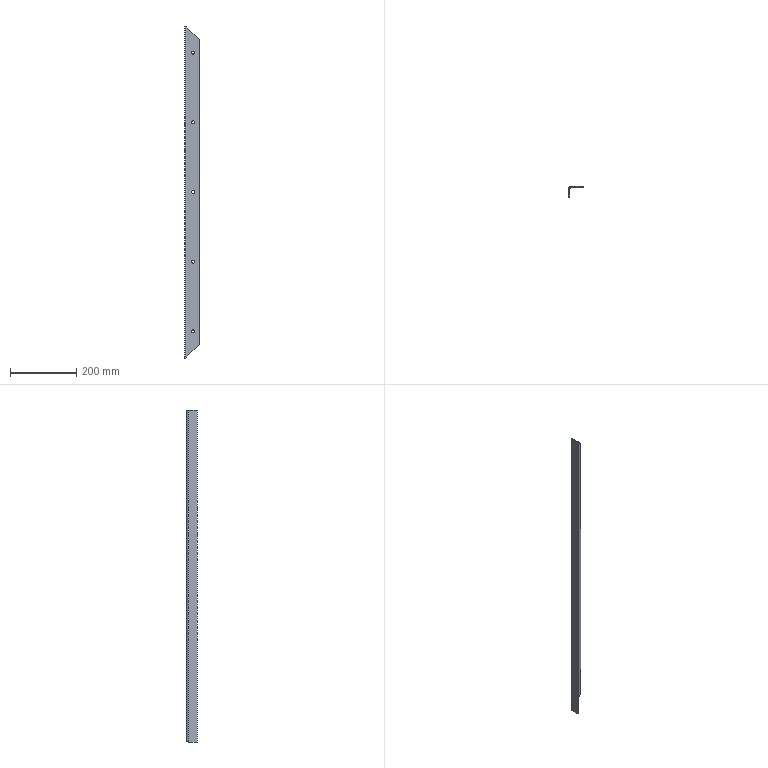Part | STEP file | 750038391 | 1 solid | 24 faces | box 43 x 33 x 1000 mm | volume 207432 mm3 | cylinder 12 | plane 10 | spline 2 | commonest cylinder face diameters 9 x10 6 x1 12 x1
STEP:
#1=CARTESIAN_POINT('',(22.,0.,415.5));
#2=VERTEX_POINT('',#1);
#3=CARTESIAN_POINT('',(22.,0.,424.5));
#4=VERTEX_POINT('',#3);
#5=CARTESIAN_POINT('',(22.,0.,420.));
#6=DIRECTION('',(0.,1.,0.));
#7=DIRECTION('',(0.,0.,1.));
#8=AXIS2_PLACEMENT_3D('',#5,#6,#7);
#9=CIRCLE('',#8,4.5);
#10=EDGE_CURVE('',#2,#4,#9,.T.);
#11=ORIENTED_EDGE('',*,*,#10,.F.);
#12=CARTESIAN_POINT('',(22.,3.,415.5));
#13=VERTEX_POINT('',#12);
#14=CARTESIAN_POINT('',(22.,-998.468,415.5));
#15=DIRECTION('',(0.,1.,0.));
#16=VECTOR('',#15,1000.);
#17=LINE('',#14,#16);
#18=EDGE_CURVE('',#2,#13,#17,.T.);
#19=ORIENTED_EDGE('',*,*,#18,.T.);
#20=CARTESIAN_POINT('',(22.,3.,424.5));
#21=VERTEX_POINT('',#20);
#22=CARTESIAN_POINT('',(22.,3.,420.));
#23=DIRECTION('',(0.,1.,0.));
#24=DIRECTION('',(0.,0.,1.));
#25=AXIS2_PLACEMENT_3D('',#22,#23,#24);
#26=CIRCLE('',#25,4.5);
#27=EDGE_CURVE('',#13,#21,#26,.T.);
#28=ORIENTED_EDGE('',*,*,#27,.T.);
#29=CARTESIAN_POINT('',(22.,-998.468,424.5));
#30=DIRECTION('',(0.,1.,0.));
#31=VECTOR('',#30,1000.);
#32=LINE('',#29,#31);
#33=EDGE_CURVE('',#4,#21,#32,.T.);
#34=ORIENTED_EDGE('',*,*,#33,.F.);
#35=EDGE_LOOP('',(#11,#19,#28,#34));
#36=FACE_OUTER_BOUND('',#35,.T.);
#37=CARTESIAN_POINT('',(22.,-998.468,420.));
#38=DIRECTION('',(0.,1.,0.));
#39=DIRECTION('',(0.,0.,1.));
#40=AXIS2_PLACEMENT_3D('',#37,#38,#39);
#41=CYLINDRICAL_SURFACE('',#40,4.5);
#42=ADVANCED_FACE('',(#36),#41,.F.);
#43=CARTESIAN_POINT('',(22.,0.,205.5));
#44=VERTEX_POINT('',#43);
#45=CARTESIAN_POINT('',(22.,0.,214.5));
#46=VERTEX_POINT('',#45);
#47=CARTESIAN_POINT('',(22.,0.,210.));
#48=DIRECTION('',(0.,1.,0.));
#49=DIRECTION('',(0.,0.,1.));
#50=AXIS2_PLACEMENT_3D('',#47,#48,#49);
#51=CIRCLE('',#50,4.5);
#52=EDGE_CURVE('',#44,#46,#51,.T.);
#53=ORIENTED_EDGE('',*,*,#52,.F.);
#54=CARTESIAN_POINT('',(22.,3.,205.5));
#55=VERTEX_POINT('',#54);
#56=CARTESIAN_POINT('',(22.,-998.468,205.5));
#57=DIRECTION('',(0.,1.,0.));
#58=VECTOR('',#57,1000.);
#59=LINE('',#56,#58);
#60=EDGE_CURVE('',#44,#55,#59,.T.);
#61=ORIENTED_EDGE('',*,*,#60,.T.);
#62=CARTESIAN_POINT('',(22.,3.,214.5));
#63=VERTEX_POINT('',#62);
#64=CARTESIAN_POINT('',(22.,3.,210.));
#65=DIRECTION('',(0.,1.,0.));
#66=DIRECTION('',(0.,0.,1.));
#67=AXIS2_PLACEMENT_3D('',#64,#65,#66);
#68=CIRCLE('',#67,4.5);
#69=EDGE_CURVE('',#55,#63,#68,.T.);
#70=ORIENTED_EDGE('',*,*,#69,.T.);
#71=CARTESIAN_POINT('',(22.,-998.468,214.5));
#72=DIRECTION('',(0.,1.,0.));
#73=VECTOR('',#72,1000.);
#74=LINE('',#71,#73);
#75=EDGE_CURVE('',#46,#63,#74,.T.);
#76=ORIENTED_EDGE('',*,*,#75,.F.);
#77=EDGE_LOOP('',(#53,#61,#70,#76));
#78=FACE_OUTER_BOUND('',#77,.T.);
#79=CARTESIAN_POINT('',(22.,-998.468,210.));
#80=DIRECTION('',(0.,1.,0.));
#81=DIRECTION('',(0.,0.,1.));
#82=AXIS2_PLACEMENT_3D('',#79,#80,#81);
#83=CYLINDRICAL_SURFACE('',#82,4.5);
#84=ADVANCED_FACE('',(#78),#83,.F.);
#85=CARTESIAN_POINT('',(22.,0.,-4.5));
#86=VERTEX_POINT('',#85);
#87=CARTESIAN_POINT('',(22.,0.,4.5));
#88=VERTEX_POINT('',#87);
#89=CARTESIAN_POINT('',(22.,0.,0.));
#90=DIRECTION('',(0.,1.,0.));
#91=DIRECTION('',(0.,0.,1.));
#92=AXIS2_PLACEMENT_3D('',#89,#90,#91);
#93=CIRCLE('',#92,4.5);
#94=EDGE_CURVE('',#86,#88,#93,.T.);
#95=ORIENTED_EDGE('',*,*,#94,.F.);
#96=CARTESIAN_POINT('',(22.,3.,-4.5));
#97=VERTEX_POINT('',#96);
#98=CARTESIAN_POINT('',(22.,-998.468,-4.5));
#99=DIRECTION('',(0.,1.,0.));
#100=VECTOR('',#99,1000.);
#101=LINE('',#98,#100);
#102=EDGE_CURVE('',#86,#97,#101,.T.);
#103=ORIENTED_EDGE('',*,*,#102,.T.);
#104=CARTESIAN_POINT('',(22.,3.,4.5));
#105=VERTEX_POINT('',#104);
#106=CARTESIAN_POINT('',(22.,3.,0.));
#107=DIRECTION('',(0.,1.,0.));
#108=DIRECTION('',(0.,0.,1.));
#109=AXIS2_PLACEMENT_3D('',#106,#107,#108);
#110=CIRCLE('',#109,4.5);
#111=EDGE_CURVE('',#97,#105,#110,.T.);
#112=ORIENTED_EDGE('',*,*,#111,.T.);
#113=CARTESIAN_POINT('',(22.,-998.468,4.5));
#114=DIRECTION('',(0.,1.,0.));
#115=VECTOR('',#114,1000.);
#116=LINE('',#113,#115);
#117=EDGE_CURVE('',#88,#105,#116,.T.);
#118=ORIENTED_EDGE('',*,*,#117,.F.);
#119=EDGE_LOOP('',(#95,#103,#112,#118));
#120=FACE_OUTER_BOUND('',#119,.T.);
#121=CARTESIAN_POINT('',(22.,-998.468,0.));
#122=DIRECTION('',(0.,1.,0.));
#123=DIRECTION('',(0.,0.,1.));
#124=AXIS2_PLACEMENT_3D('',#121,#122,#123);
#125=CYLINDRICAL_SURFACE('',#124,4.5);
#126=ADVANCED_FACE('',(#120),#125,.F.);
#127=CARTESIAN_POINT('',(22.,0.,-214.5));
#128=VERTEX_POINT('',#127);
#129=CARTESIAN_POINT('',(22.,0.,-205.5));
#130=VERTEX_POINT('',#129);
#131=CARTESIAN_POINT('',(22.,0.,-210.));
#132=DIRECTION('',(0.,1.,0.));
#133=DIRECTION('',(0.,0.,1.));
#134=AXIS2_PLACEMENT_3D('',#131,#132,#133);
#135=CIRCLE('',#134,4.5);
#136=EDGE_CURVE('',#128,#130,#135,.T.);
#137=ORIENTED_EDGE('',*,*,#136,.F.);
#138=CARTESIAN_POINT('',(22.,3.,-214.5));
#139=VERTEX_POINT('',#138);
#140=CARTESIAN_POINT('',(22.,-998.468,-214.5));
#141=DIRECTION('',(0.,1.,0.));
#142=VECTOR('',#141,1000.);
#143=LINE('',#140,#142);
#144=EDGE_CURVE('',#128,#139,#143,.T.);
#145=ORIENTED_EDGE('',*,*,#144,.T.);
#146=CARTESIAN_POINT('',(22.,3.,-205.5));
#147=VERTEX_POINT('',#146);
#148=CARTESIAN_POINT('',(22.,3.,-210.));
#149=DIRECTION('',(0.,1.,0.));
#150=DIRECTION('',(0.,0.,1.));
#151=AXIS2_PLACEMENT_3D('',#148,#149,#150);
#152=CIRCLE('',#151,4.5);
#153=EDGE_CURVE('',#139,#147,#152,.T.);
#154=ORIENTED_EDGE('',*,*,#153,.T.);
#155=CARTESIAN_POINT('',(22.,-998.468,-205.5));
#156=DIRECTION('',(0.,1.,0.));
#157=VECTOR('',#156,1000.);
#158=LINE('',#155,#157);
#159=EDGE_CURVE('',#130,#147,#158,.T.);
#160=ORIENTED_EDGE('',*,*,#159,.F.);
#161=EDGE_LOOP('',(#137,#145,#154,#160));
#162=FACE_OUTER_BOUND('',#161,.T.);
#163=CARTESIAN_POINT('',(22.,-998.468,-210.));
#164=DIRECTION('',(0.,1.,0.));
#165=DIRECTION('',(0.,0.,1.));
#166=AXIS2_PLACEMENT_3D('',#163,#164,#165);
#167=CYLINDRICAL_SURFACE('',#166,4.5);
#168=ADVANCED_FACE('',(#162),#167,.F.);
#169=CARTESIAN_POINT('',(22.,0.,-424.5));
#170=VERTEX_POINT('',#169);
#171=CARTESIAN_POINT('',(22.,0.,-415.5));
#172=VERTEX_POINT('',#171);
#173=CARTESIAN_POINT('',(22.,0.,-420.));
#174=DIRECTION('',(0.,1.,0.));
#175=DIRECTION('',(0.,0.,1.));
#176=AXIS2_PLACEMENT_3D('',#173,#174,#175);
#177=CIRCLE('',#176,4.5);
#178=EDGE_CURVE('',#170,#172,#177,.T.);
#179=ORIENTED_EDGE('',*,*,#178,.F.);
#180=CARTESIAN_POINT('',(22.,3.,-424.5));
#181=VERTEX_POINT('',#180);
#182=CARTESIAN_POINT('',(22.,-998.468,-424.5));
#183=DIRECTION('',(0.,1.,0.));
#184=VECTOR('',#183,1000.);
#185=LINE('',#182,#184);
#186=EDGE_CURVE('',#170,#181,#185,.T.);
#187=ORIENTED_EDGE('',*,*,#186,.T.);
#188=CARTESIAN_POINT('',(22.,3.,-415.5));
#189=VERTEX_POINT('',#188);
#190=CARTESIAN_POINT('',(22.,3.,-420.));
#191=DIRECTION('',(0.,1.,0.));
#192=DIRECTION('',(0.,0.,1.));
#193=AXIS2_PLACEMENT_3D('',#190,#191,#192);
#194=CIRCLE('',#193,4.5);
#195=EDGE_CURVE('',#181,#189,#194,.T.);
#196=ORIENTED_EDGE('',*,*,#195,.T.);
#197=CARTESIAN_POINT('',(22.,-998.468,-415.5));
#198=DIRECTION('',(0.,1.,0.));
#199=VECTOR('',#198,1000.);
#200=LINE('',#197,#199);
#201=EDGE_CURVE('',#172,#189,#200,.T.);
#202=ORIENTED_EDGE('',*,*,#201,.F.);
#203=EDGE_LOOP('',(#179,#187,#196,#202));
#204=FACE_OUTER_BOUND('',#203,.T.);
#205=CARTESIAN_POINT('',(22.,-998.468,-420.));
#206=DIRECTION('',(0.,1.,0.));
#207=DIRECTION('',(0.,0.,1.));
#208=AXIS2_PLACEMENT_3D('',#205,#206,#207);
#209=CYLINDRICAL_SURFACE('',#208,4.5);
#210=ADVANCED_FACE('',(#204),#209,.F.);
#211=CARTESIAN_POINT('',(40.,3.,-460.));
#212=VERTEX_POINT('',#211);
#213=CARTESIAN_POINT('',(40.,3.,460.));
#214=VERTEX_POINT('',#213);
#215=CARTESIAN_POINT('',(40.,3.,500.));
#216=DIRECTION('',(0.,0.,1.));
#217=VECTOR('',#216,1000.);
#218=LINE('',#215,#217);
#219=EDGE_CURVE('',#212,#214,#218,.T.);
#220=ORIENTED_EDGE('',*,*,#219,.F.);
#221=CARTESIAN_POINT('',(3.,3.,-497.));
#222=VERTEX_POINT('',#221);
#223=CARTESIAN_POINT('',(3.,3.,-497.));
#224=DIRECTION('',(0.7071,0.,0.7071));
#225=VECTOR('',#224,1000.);
#226=LINE('',#223,#225);
#227=EDGE_CURVE('',#222,#212,#226,.T.);
#228=ORIENTED_EDGE('',*,*,#227,.F.);
#229=CARTESIAN_POINT('',(3.,3.,497.));
#230=VERTEX_POINT('',#229);
#231=CARTESIAN_POINT('',(3.,3.,500.));
#232=DIRECTION('',(0.,0.,-1.));
#233=VECTOR('',#232,1000.);
#234=LINE('',#231,#233);
#235=EDGE_CURVE('',#230,#222,#234,.T.);
#236=ORIENTED_EDGE('',*,*,#235,.F.);
#237=CARTESIAN_POINT('',(40.,3.,460.));
#238=DIRECTION('',(-0.7071,0.,0.7071));
#239=VECTOR('',#238,1000.);
#240=LINE('',#237,#239);
#241=EDGE_CURVE('',#214,#230,#240,.T.);
#242=ORIENTED_EDGE('',*,*,#241,.F.);
#243=EDGE_LOOP('',(#220,#228,#236,#242));
#244=FACE_OUTER_BOUND('',#243,.T.);
#245=CARTESIAN_POINT('',(22.,3.,420.));
#246=DIRECTION('',(0.,1.,0.));
#247=DIRECTION('',(0.,0.,1.));
#248=AXIS2_PLACEMENT_3D('',#245,#246,#247);
#249=CIRCLE('',#248,4.5);
#250=EDGE_CURVE('',#21,#13,#249,.T.);
#251=ORIENTED_EDGE('',*,*,#250,.F.);
#252=ORIENTED_EDGE('',*,*,#27,.F.);
#253=EDGE_LOOP('',(#251,#252));
#254=FACE_BOUND('',#253,.T.);
#255=CARTESIAN_POINT('',(22.,3.,210.));
#256=DIRECTION('',(0.,1.,0.));
#257=DIRECTION('',(0.,0.,1.));
#258=AXIS2_PLACEMENT_3D('',#255,#256,#257);
#259=CIRCLE('',#258,4.5);
#260=EDGE_CURVE('',#63,#55,#259,.T.);
#261=ORIENTED_EDGE('',*,*,#260,.F.);
#262=ORIENTED_EDGE('',*,*,#69,.F.);
#263=EDGE_LOOP('',(#261,#262));
#264=FACE_BOUND('',#263,.T.);
#265=CARTESIAN_POINT('',(22.,3.,0.));
#266=DIRECTION('',(0.,1.,0.));
#267=DIRECTION('',(0.,0.,1.));
#268=AXIS2_PLACEMENT_3D('',#265,#266,#267);
#269=CIRCLE('',#268,4.5);
#270=EDGE_CURVE('',#105,#97,#269,.T.);
#271=ORIENTED_EDGE('',*,*,#270,.F.);
#272=ORIENTED_EDGE('',*,*,#111,.F.);
#273=EDGE_LOOP('',(#271,#272));
#274=FACE_BOUND('',#273,.T.);
#275=CARTESIAN_POINT('',(22.,3.,-210.));
#276=DIRECTION('',(0.,1.,0.));
#277=DIRECTION('',(0.,0.,1.));
#278=AXIS2_PLACEMENT_3D('',#275,#276,#277);
#279=CIRCLE('',#278,4.5);
#280=EDGE_CURVE('',#147,#139,#279,.T.);
#281=ORIENTED_EDGE('',*,*,#280,.F.);
#282=ORIENTED_EDGE('',*,*,#153,.F.);
#283=EDGE_LOOP('',(#281,#282));
#284=FACE_BOUND('',#283,.T.);
#285=CARTESIAN_POINT('',(22.,3.,-420.));
#286=DIRECTION('',(0.,1.,0.));
#287=DIRECTION('',(0.,0.,1.));
#288=AXIS2_PLACEMENT_3D('',#285,#286,#287);
#289=CIRCLE('',#288,4.5);
#290=EDGE_CURVE('',#189,#181,#289,.T.);
#291=ORIENTED_EDGE('',*,*,#290,.F.);
#292=ORIENTED_EDGE('',*,*,#195,.F.);
#293=EDGE_LOOP('',(#291,#292));
#294=FACE_BOUND('',#293,.T.);
#295=CARTESIAN_POINT('',(40.,3.,500.));
#296=DIRECTION('',(0.,-1.,0.));
#297=DIRECTION('',(0.,0.,-1.));
#298=AXIS2_PLACEMENT_3D('',#295,#296,#297);
#299=PLANE('',#298);
#300=ADVANCED_FACE('',(#244,#254,#264,#274,#284,#294),#299,.F.);
#301=CARTESIAN_POINT('',(40.,0.,460.));
#302=VERTEX_POINT('',#301);
#303=CARTESIAN_POINT('',(40.,0.,460.));
#304=DIRECTION('',(0.,1.,0.));
#305=VECTOR('',#304,1000.);
#306=LINE('',#303,#305);
#307=EDGE_CURVE('',#302,#214,#306,.T.);
#308=ORIENTED_EDGE('',*,*,#307,.T.);
#309=ORIENTED_EDGE('',*,*,#241,.T.);
#310=CARTESIAN_POINT('',(3.,0.,497.));
#311=VERTEX_POINT('',#310);
#312=CARTESIAN_POINT('',(3.,0.,497.));
#313=DIRECTION('',(0.,-1.,0.));
#314=VECTOR('',#313,1000.);
#315=LINE('',#312,#314);
#316=EDGE_CURVE('',#230,#311,#315,.T.);
#317=ORIENTED_EDGE('',*,*,#316,.T.);
#318=CARTESIAN_POINT('',(20.,0.,480.));
#319=DIRECTION('',(0.7071,0.,-0.7071));
#320=VECTOR('',#319,1000.);
#321=LINE('',#318,#320);
#322=EDGE_CURVE('',#311,#302,#321,.T.);
#323=ORIENTED_EDGE('',*,*,#322,.T.);
#324=EDGE_LOOP('',(#308,#309,#317,#323));
#325=FACE_OUTER_BOUND('',#324,.T.);
#326=CARTESIAN_POINT('',(20.,0.,480.));
#327=DIRECTION('',(0.7071,0.,0.7071));
#328=DIRECTION('',(0.7071,0.,-0.7071));
#329=AXIS2_PLACEMENT_3D('',#326,#327,#328);
#330=PLANE('',#329);
#331=ADVANCED_FACE('',(#325),#330,.T.);
#332=ORIENTED_EDGE('',*,*,#307,.F.);
#333=CARTESIAN_POINT('',(40.,0.,-460.));
#334=VERTEX_POINT('',#333);
#335=CARTESIAN_POINT('',(40.,0.,500.));
#336=DIRECTION('',(0.,0.,1.));
#337=VECTOR('',#336,1000.);
#338=LINE('',#335,#337);
#339=EDGE_CURVE('',#334,#302,#338,.T.);
#340=ORIENTED_EDGE('',*,*,#339,.F.);
#341=CARTESIAN_POINT('',(40.,0.,-460.));
#342=DIRECTION('',(0.,-1.,0.));
#343=VECTOR('',#342,1000.);
#344=LINE('',#341,#343);
#345=EDGE_CURVE('',#212,#334,#344,.T.);
#346=ORIENTED_EDGE('',*,*,#345,.F.);
#347=ORIENTED_EDGE('',*,*,#219,.T.);
#348=EDGE_LOOP('',(#332,#340,#346,#347));
#349=FACE_OUTER_BOUND('',#348,.T.);
#350=CARTESIAN_POINT('',(40.,0.,500.));
#351=DIRECTION('',(-1.,0.,0.));
#352=DIRECTION('',(0.,0.,1.));
#353=AXIS2_PLACEMENT_3D('',#350,#351,#352);
#354=PLANE('',#353);
#355=ADVANCED_FACE('',(#349),#354,.F.);
#356=CARTESIAN_POINT('',(3.,0.,-497.));
#357=VERTEX_POINT('',#356);
#358=CARTESIAN_POINT('',(3.,0.,-497.));
#359=DIRECTION('',(0.,1.,0.));
#360=VECTOR('',#359,1000.);
#361=LINE('',#358,#360);
#362=EDGE_CURVE('',#357,#222,#361,.T.);
#363=ORIENTED_EDGE('',*,*,#362,.T.);
#364=ORIENTED_EDGE('',*,*,#227,.T.);
#365=ORIENTED_EDGE('',*,*,#345,.T.);
#366=CARTESIAN_POINT('',(520.,0.,20.));
#367=DIRECTION('',(-0.7071,0.,-0.7071));
#368=VECTOR('',#367,1000.);
#369=LINE('',#366,#368);
#370=EDGE_CURVE('',#334,#357,#369,.T.);
#371=ORIENTED_EDGE('',*,*,#370,.T.);
#372=EDGE_LOOP('',(#363,#364,#365,#371));
#373=FACE_OUTER_BOUND('',#372,.T.);
#374=CARTESIAN_POINT('',(520.,0.,20.));
#375=DIRECTION('',(0.7071,0.,-0.7071));
#376=DIRECTION('',(-0.7071,0.,-0.7071));
#377=AXIS2_PLACEMENT_3D('',#374,#375,#376);
#378=PLANE('',#377);
#379=ADVANCED_FACE('',(#373),#378,.T.);
#380=CARTESIAN_POINT('',(-3.,-3.,-500.));
#381=VERTEX_POINT('',#380);
#382=CARTESIAN_POINT('',(3.,3.,-497.));
#383=CARTESIAN_POINT('',(-1.,3.,-499.));
#384=CARTESIAN_POINT('',(-3.,0.,-500.));
#385=CARTESIAN_POINT('',(-3.,-3.,-500.));
#386=(BOUNDED_CURVE()B_SPLINE_CURVE(3,(#382,#383,#384,#385),.UNSPECIFIED.,.F.,.T.)B_SPLINE_CURVE_WITH_KNOTS((4,4),(0.,0.009933),.UNSPECIFIED.)CURVE()GEOMETRIC_REPRESENTATION_ITEM()RATIONAL_B_SPLINE_CURVE((0.5,0.5,0.6667,1.))REPRESENTATION_ITEM(''));
#387=EDGE_CURVE('',#222,#381,#386,.T.);
#388=ORIENTED_EDGE('',*,*,#387,.T.);
#389=CARTESIAN_POINT('',(-3.,-3.,500.));
#390=VERTEX_POINT('',#389);
#391=CARTESIAN_POINT('',(-3.,-3.,500.));
#392=DIRECTION('',(0.,0.,1.));
#393=VECTOR('',#392,1000.);
#394=LINE('',#391,#393);
#395=EDGE_CURVE('',#381,#390,#394,.T.);
#396=ORIENTED_EDGE('',*,*,#395,.T.);
#397=CARTESIAN_POINT('',(-3.,-3.,500.));
#398=CARTESIAN_POINT('',(-3.,0.,500.));
#399=CARTESIAN_POINT('',(-1.,3.,499.));
#400=CARTESIAN_POINT('',(3.,3.,497.));
#401=(BOUNDED_CURVE()B_SPLINE_CURVE(3,(#397,#398,#399,#400),.UNSPECIFIED.,.F.,.T.)B_SPLINE_CURVE_WITH_KNOTS((4,4),(0.,0.009979),.UNSPECIFIED.)CURVE()GEOMETRIC_REPRESENTATION_ITEM()RATIONAL_B_SPLINE_CURVE((1.,0.6667,0.5,0.5))REPRESENTATION_ITEM(''));
#402=EDGE_CURVE('',#390,#230,#401,.T.);
#403=ORIENTED_EDGE('',*,*,#402,.T.);
#404=ORIENTED_EDGE('',*,*,#235,.T.);
#405=EDGE_LOOP('',(#388,#396,#403,#404));
#406=FACE_OUTER_BOUND('',#405,.T.);
#407=CARTESIAN_POINT('',(3.,-3.,500.));
#408=DIRECTION('',(0.,0.,-1.));
#409=DIRECTION('',(-1.,0.,0.));
#410=AXIS2_PLACEMENT_3D('',#407,#408,#409);
#411=CYLINDRICAL_SURFACE('',#410,6.);
#412=ADVANCED_FACE('',(#406),#411,.T.);
#413=ORIENTED_EDGE('',*,*,#18,.F.);
#414=CARTESIAN_POINT('',(22.,0.,420.));
#415=DIRECTION('',(0.,1.,0.));
#416=DIRECTION('',(0.,0.,1.));
#417=AXIS2_PLACEMENT_3D('',#414,#415,#416);
#418=CIRCLE('',#417,4.5);
#419=EDGE_CURVE('',#4,#2,#418,.T.);
#420=ORIENTED_EDGE('',*,*,#419,.F.);
#421=ORIENTED_EDGE('',*,*,#33,.T.);
#422=ORIENTED_EDGE('',*,*,#250,.T.);
#423=EDGE_LOOP('',(#413,#420,#421,#422));
#424=FACE_OUTER_BOUND('',#423,.T.);
#425=CARTESIAN_POINT('',(22.,-998.468,420.));
#426=DIRECTION('',(0.,1.,0.));
#427=DIRECTION('',(0.,0.,1.));
#428=AXIS2_PLACEMENT_3D('',#425,#426,#427);
#429=CYLINDRICAL_SURFACE('',#428,4.5);
#430=ADVANCED_FACE('',(#424),#429,.F.);
#431=ORIENTED_EDGE('',*,*,#60,.F.);
#432=CARTESIAN_POINT('',(22.,0.,210.));
#433=DIRECTION('',(0.,1.,0.));
#434=DIRECTION('',(0.,0.,1.));
#435=AXIS2_PLACEMENT_3D('',#432,#433,#434);
#436=CIRCLE('',#435,4.5);
#437=EDGE_CURVE('',#46,#44,#436,.T.);
#438=ORIENTED_EDGE('',*,*,#437,.F.);
#439=ORIENTED_EDGE('',*,*,#75,.T.);
#440=ORIENTED_EDGE('',*,*,#260,.T.);
#441=EDGE_LOOP('',(#431,#438,#439,#440));
#442=FACE_OUTER_BOUND('',#441,.T.);
#443=CARTESIAN_POINT('',(22.,-998.468,210.));
#444=DIRECTION('',(0.,1.,0.));
#445=DIRECTION('',(0.,0.,1.));
#446=AXIS2_PLACEMENT_3D('',#443,#444,#445);
#447=CYLINDRICAL_SURFACE('',#446,4.5);
#448=ADVANCED_FACE('',(#442),#447,.F.);
#449=ORIENTED_EDGE('',*,*,#102,.F.);
#450=CARTESIAN_POINT('',(22.,0.,0.));
#451=DIRECTION('',(0.,1.,0.));
#452=DIRECTION('',(0.,0.,1.));
#453=AXIS2_PLACEMENT_3D('',#450,#451,#452);
#454=CIRCLE('',#453,4.5);
#455=EDGE_CURVE('',#88,#86,#454,.T.);
#456=ORIENTED_EDGE('',*,*,#455,.F.);
#457=ORIENTED_EDGE('',*,*,#117,.T.);
#458=ORIENTED_EDGE('',*,*,#270,.T.);
#459=EDGE_LOOP('',(#449,#456,#457,#458));
#460=FACE_OUTER_BOUND('',#459,.T.);
#461=CARTESIAN_POINT('',(22.,-998.468,0.));
#462=DIRECTION('',(0.,1.,0.));
#463=DIRECTION('',(0.,0.,1.));
#464=AXIS2_PLACEMENT_3D('',#461,#462,#463);
#465=CYLINDRICAL_SURFACE('',#464,4.5);
#466=ADVANCED_FACE('',(#460),#465,.F.);
#467=ORIENTED_EDGE('',*,*,#144,.F.);
#468=CARTESIAN_POINT('',(22.,0.,-210.));
#469=DIRECTION('',(0.,1.,0.));
#470=DIRECTION('',(0.,0.,1.));
#471=AXIS2_PLACEMENT_3D('',#468,#469,#470);
#472=CIRCLE('',#471,4.5);
#473=EDGE_CURVE('',#130,#128,#472,.T.);
#474=ORIENTED_EDGE('',*,*,#473,.F.);
#475=ORIENTED_EDGE('',*,*,#159,.T.);
#476=ORIENTED_EDGE('',*,*,#280,.T.);
#477=EDGE_LOOP('',(#467,#474,#475,#476));
#478=FACE_OUTER_BOUND('',#477,.T.);
#479=CARTESIAN_POINT('',(22.,-998.468,-210.));
#480=DIRECTION('',(0.,1.,0.));
#481=DIRECTION('',(0.,0.,1.));
#482=AXIS2_PLACEMENT_3D('',#479,#480,#481);
#483=CYLINDRICAL_SURFACE('',#482,4.5);
#484=ADVANCED_FACE('',(#478),#483,.F.);
#485=ORIENTED_EDGE('',*,*,#186,.F.);
#486=CARTESIAN_POINT('',(22.,0.,-420.));
#487=DIRECTION('',(0.,1.,0.));
#488=DIRECTION('',(0.,0.,1.));
#489=AXIS2_PLACEMENT_3D('',#486,#487,#488);
#490=CIRCLE('',#489,4.5);
#491=EDGE_CURVE('',#172,#170,#490,.T.);
#492=ORIENTED_EDGE('',*,*,#491,.F.);
#493=ORIENTED_EDGE('',*,*,#201,.T.);
#494=ORIENTED_EDGE('',*,*,#290,.T.);
#495=EDGE_LOOP('',(#485,#492,#493,#494));
#496=FACE_OUTER_BOUND('',#495,.T.);
#497=CARTESIAN_POINT('',(22.,-998.468,-420.));
#498=DIRECTION('',(0.,1.,0.));
#499=DIRECTION('',(0.,0.,1.));
#500=AXIS2_PLACEMENT_3D('',#497,#498,#499);
#501=CYLINDRICAL_SURFACE('',#500,4.5);
#502=ADVANCED_FACE('',(#496),#501,.F.);
#503=CARTESIAN_POINT('',(3.,0.,500.));
#504=DIRECTION('',(0.,0.,-1.));
#505=VECTOR('',#504,1000.);
#506=LINE('',#503,#505);
#507=EDGE_CURVE('',#311,#357,#506,.T.);
#508=ORIENTED_EDGE('',*,*,#507,.T.);
#509=ORIENTED_EDGE('',*,*,#370,.F.);
#510=ORIENTED_EDGE('',*,*,#339,.T.);
#511=ORIENTED_EDGE('',*,*,#322,.F.);
#512=EDGE_LOOP('',(#508,#509,#510,#511));
#513=FACE_OUTER_BOUND('',#512,.T.);
#514=ORIENTED_EDGE('',*,*,#419,.T.);
#515=ORIENTED_EDGE('',*,*,#10,.T.);
#516=EDGE_LOOP('',(#514,#515));
#517=FACE_BOUND('',#516,.T.);
#518=ORIENTED_EDGE('',*,*,#437,.T.);
#519=ORIENTED_EDGE('',*,*,#52,.T.);
#520=EDGE_LOOP('',(#518,#519));
#521=FACE_BOUND('',#520,.T.);
#522=ORIENTED_EDGE('',*,*,#455,.T.);
#523=ORIENTED_EDGE('',*,*,#94,.T.);
#524=EDGE_LOOP('',(#522,#523));
#525=FACE_BOUND('',#524,.T.);
#526=ORIENTED_EDGE('',*,*,#473,.T.);
#527=ORIENTED_EDGE('',*,*,#136,.T.);
#528=EDGE_LOOP('',(#526,#527));
#529=FACE_BOUND('',#528,.T.);
#530=ORIENTED_EDGE('',*,*,#491,.T.);
#531=ORIENTED_EDGE('',*,*,#178,.T.);
#532=EDGE_LOOP('',(#530,#531));
#533=FACE_BOUND('',#532,.T.);
#534=CARTESIAN_POINT('',(40.,0.,500.));
#535=DIRECTION('',(0.,-1.,0.));
#536=DIRECTION('',(0.,0.,-1.));
#537=AXIS2_PLACEMENT_3D('',#534,#535,#536);
#538=PLANE('',#537);
#539=ADVANCED_FACE('',(#513,#517,#521,#525,#529,#533),#538,.T.);
#540=CARTESIAN_POINT('',(0.,-3.,500.));
#541=VERTEX_POINT('',#540);
#542=CARTESIAN_POINT('',(3.,0.,497.));
#543=CARTESIAN_POINT('',(1.,0.,499.));
#544=CARTESIAN_POINT('',(0.,-1.5,500.));
#545=CARTESIAN_POINT('',(0.,-3.,500.));
#546=(BOUNDED_CURVE()B_SPLINE_CURVE(3,(#542,#543,#544,#545),.UNSPECIFIED.,.F.,.F.)B_SPLINE_CURVE_WITH_KNOTS((4,4),(0.,0.005677),.UNSPECIFIED.)CURVE()GEOMETRIC_REPRESENTATION_ITEM()RATIONAL_B_SPLINE_CURVE((0.5,0.5,0.6667,1.))REPRESENTATION_ITEM(''));
#547=EDGE_CURVE('',#311,#541,#546,.T.);
#548=ORIENTED_EDGE('',*,*,#547,.F.);
#549=ORIENTED_EDGE('',*,*,#316,.F.);
#550=ORIENTED_EDGE('',*,*,#402,.F.);
#551=CARTESIAN_POINT('',(-1.5,-3.,500.));
#552=DIRECTION('',(-1.,0.,0.));
#553=VECTOR('',#552,1000.);
#554=LINE('',#551,#553);
#555=EDGE_CURVE('',#541,#390,#554,.T.);
#556=ORIENTED_EDGE('',*,*,#555,.F.);
#557=EDGE_LOOP('',(#548,#549,#550,#556));
#558=FACE_OUTER_BOUND('',#557,.T.);
#559=CARTESIAN_POINT('',(6.,-3.,494.));
#560=CARTESIAN_POINT('',(7.,-3.,494.));
#561=CARTESIAN_POINT('',(8.,-3.,494.));
#562=CARTESIAN_POINT('',(9.,-3.,494.));
#563=CARTESIAN_POINT('',(6.,3.,494.));
#564=CARTESIAN_POINT('',(7.,5.,494.));
#565=CARTESIAN_POINT('',(8.,7.,494.));
#566=CARTESIAN_POINT('',(9.,9.,494.));
#567=CARTESIAN_POINT('',(0.,3.,500.));
#568=CARTESIAN_POINT('',(-1.,5.,500.));
#569=CARTESIAN_POINT('',(-2.,7.,500.));
#570=CARTESIAN_POINT('',(-3.,9.,500.));
#571=CARTESIAN_POINT('',(0.,-3.,500.));
#572=CARTESIAN_POINT('',(-1.,-3.,500.));
#573=CARTESIAN_POINT('',(-2.,-3.,500.));
#574=CARTESIAN_POINT('',(-3.,-3.,500.));
#575=CARTESIAN_POINT('',(0.,-9.,500.));
#576=CARTESIAN_POINT('',(-1.,-11.,500.));
#577=CARTESIAN_POINT('',(-2.,-13.,500.));
#578=CARTESIAN_POINT('',(-3.,-15.,500.));
#579=CARTESIAN_POINT('',(6.,-9.,494.));
#580=CARTESIAN_POINT('',(7.,-11.,494.));
#581=CARTESIAN_POINT('',(8.,-13.,494.));
#582=CARTESIAN_POINT('',(9.,-15.,494.));
#583=CARTESIAN_POINT('',(6.,-3.,494.));
#584=CARTESIAN_POINT('',(7.,-3.,494.));
#585=CARTESIAN_POINT('',(8.,-3.,494.));
#586=CARTESIAN_POINT('',(9.,-3.,494.));
#587=(BOUNDED_SURFACE()B_SPLINE_SURFACE(3,3,((#559,#560,#561,#562),(#563,#564,#565,#566),(#567,#568,#569,#570),(#571,#572,#573,#574),(#575,#576,#577,#578),(#579,#580,#581,#582),(#583,#584,#585,#586)),.UNSPECIFIED.,.T.,.F.,.T.)B_SPLINE_SURFACE_WITH_KNOTS((4,3,4),(4,4),(0.,0.5,1.),(0.,1.),.UNSPECIFIED.)GEOMETRIC_REPRESENTATION_ITEM()RATIONAL_B_SPLINE_SURFACE(((1.,1.,1.,1.),(0.3333,0.3333,0.3333,0.3333),(0.3333,0.3333,0.3333,0.3333),(1.,1.,1.,1.),(0.3333,0.3333,0.3333,0.3333),(0.3333,0.3333,0.3333,0.3333),(1.,1.,1.,1.)))REPRESENTATION_ITEM('')SURFACE());
#588=ADVANCED_FACE('',(#558),#587,.F.);
#589=CARTESIAN_POINT('',(0.,-3.,-500.));
#590=VERTEX_POINT('',#589);
#591=CARTESIAN_POINT('',(0.,-3.,-500.));
#592=CARTESIAN_POINT('',(0.,-1.5,-500.));
#593=CARTESIAN_POINT('',(1.,0.,-499.));
#594=CARTESIAN_POINT('',(3.,0.,-497.));
#595=(BOUNDED_CURVE()B_SPLINE_CURVE(3,(#591,#592,#593,#594),.UNSPECIFIED.,.F.,.T.)B_SPLINE_CURVE_WITH_KNOTS((4,4),(0.,0.005708),.UNSPECIFIED.)CURVE()GEOMETRIC_REPRESENTATION_ITEM()RATIONAL_B_SPLINE_CURVE((1.,0.6667,0.5,0.5))REPRESENTATION_ITEM(''));
#596=EDGE_CURVE('',#590,#357,#595,.T.);
#597=ORIENTED_EDGE('',*,*,#596,.F.);
#598=CARTESIAN_POINT('',(-1.5,-3.,-500.));
#599=DIRECTION('',(1.,0.,0.));
#600=VECTOR('',#599,1000.);
#601=LINE('',#598,#600);
#602=EDGE_CURVE('',#381,#590,#601,.T.);
#603=ORIENTED_EDGE('',*,*,#602,.F.);
#604=ORIENTED_EDGE('',*,*,#387,.F.);
#605=ORIENTED_EDGE('',*,*,#362,.F.);
#606=EDGE_LOOP('',(#597,#603,#604,#605));
#607=FACE_OUTER_BOUND('',#606,.T.);
#608=CARTESIAN_POINT('',(0.,-3.,-500.));
#609=CARTESIAN_POINT('',(-1.,-3.,-500.));
#610=CARTESIAN_POINT('',(-2.,-3.,-500.));
#611=CARTESIAN_POINT('',(-3.,-3.,-500.));
#612=CARTESIAN_POINT('',(0.,3.,-500.));
#613=CARTESIAN_POINT('',(-1.,5.,-500.));
#614=CARTESIAN_POINT('',(-2.,7.,-500.));
#615=CARTESIAN_POINT('',(-3.,9.,-500.));
#616=CARTESIAN_POINT('',(6.,3.,-494.));
#617=CARTESIAN_POINT('',(7.,5.,-494.));
#618=CARTESIAN_POINT('',(8.,7.,-494.));
#619=CARTESIAN_POINT('',(9.,9.,-494.));
#620=CARTESIAN_POINT('',(6.,-3.,-494.));
#621=CARTESIAN_POINT('',(7.,-3.,-494.));
#622=CARTESIAN_POINT('',(8.,-3.,-494.));
#623=CARTESIAN_POINT('',(9.,-3.,-494.));
#624=CARTESIAN_POINT('',(6.,-9.,-494.));
#625=CARTESIAN_POINT('',(7.,-11.,-494.));
#626=CARTESIAN_POINT('',(8.,-13.,-494.));
#627=CARTESIAN_POINT('',(9.,-15.,-494.));
#628=CARTESIAN_POINT('',(0.,-9.,-500.));
#629=CARTESIAN_POINT('',(-1.,-11.,-500.));
#630=CARTESIAN_POINT('',(-2.,-13.,-500.));
#631=CARTESIAN_POINT('',(-3.,-15.,-500.));
#632=CARTESIAN_POINT('',(0.,-3.,-500.));
#633=CARTESIAN_POINT('',(-1.,-3.,-500.));
#634=CARTESIAN_POINT('',(-2.,-3.,-500.));
#635=CARTESIAN_POINT('',(-3.,-3.,-500.));
#636=(BOUNDED_SURFACE()B_SPLINE_SURFACE(3,3,((#608,#609,#610,#611),(#612,#613,#614,#615),(#616,#617,#618,#619),(#620,#621,#622,#623),(#624,#625,#626,#627),(#628,#629,#630,#631),(#632,#633,#634,#635)),.UNSPECIFIED.,.T.,.F.,.F.)B_SPLINE_SURFACE_WITH_KNOTS((4,3,4),(4,4),(0.,0.5,1.),(0.,1.),.UNSPECIFIED.)GEOMETRIC_REPRESENTATION_ITEM()RATIONAL_B_SPLINE_SURFACE(((1.,1.,1.,1.),(0.3333,0.3333,0.3333,0.3333),(0.3333,0.3333,0.3333,0.3333),(1.,1.,1.,1.),(0.3333,0.3333,0.3333,0.3333),(0.3333,0.3333,0.3333,0.3333),(1.,1.,1.,1.)))REPRESENTATION_ITEM('')SURFACE());
#637=ADVANCED_FACE('',(#607),#636,.F.);
#638=CARTESIAN_POINT('',(-3.,-30.,500.));
#639=VERTEX_POINT('',#638);
#640=CARTESIAN_POINT('',(-3.,-30.,-500.));
#641=VERTEX_POINT('',#640);
#642=CARTESIAN_POINT('',(-3.,-30.,500.));
#643=DIRECTION('',(0.,0.,-1.));
#644=VECTOR('',#643,1000.);
#645=LINE('',#642,#644);
#646=EDGE_CURVE('',#639,#641,#645,.T.);
#647=ORIENTED_EDGE('',*,*,#646,.F.);
#648=CARTESIAN_POINT('',(-3.,0.,500.));
#649=DIRECTION('',(0.,-1.,0.));
#650=VECTOR('',#649,1000.);
#651=LINE('',#648,#650);
#652=EDGE_CURVE('',#390,#639,#651,.T.);
#653=ORIENTED_EDGE('',*,*,#652,.F.);
#654=ORIENTED_EDGE('',*,*,#395,.F.);
#655=CARTESIAN_POINT('',(-3.,0.,-500.));
#656=DIRECTION('',(0.,1.,0.));
#657=VECTOR('',#656,1000.);
#658=LINE('',#655,#657);
#659=EDGE_CURVE('',#641,#381,#658,.T.);
#660=ORIENTED_EDGE('',*,*,#659,.F.);
#661=EDGE_LOOP('',(#647,#653,#654,#660));
#662=FACE_OUTER_BOUND('',#661,.T.);
#663=CARTESIAN_POINT('',(-3.,0.,500.));
#664=DIRECTION('',(1.,0.,0.));
#665=DIRECTION('',(0.,1.,0.));
#666=AXIS2_PLACEMENT_3D('',#663,#664,#665);
#667=PLANE('',#666);
#668=ADVANCED_FACE('',(#662),#667,.F.);
#669=ORIENTED_EDGE('',*,*,#547,.T.);
#670=CARTESIAN_POINT('',(0.,-3.,500.));
#671=DIRECTION('',(0.,0.,1.));
#672=VECTOR('',#671,1000.);
#673=LINE('',#670,#672);
#674=EDGE_CURVE('',#590,#541,#673,.T.);
#675=ORIENTED_EDGE('',*,*,#674,.F.);
#676=ORIENTED_EDGE('',*,*,#596,.T.);
#677=ORIENTED_EDGE('',*,*,#507,.F.);
#678=EDGE_LOOP('',(#669,#675,#676,#677));
#679=FACE_OUTER_BOUND('',#678,.T.);
#680=CARTESIAN_POINT('',(3.,-3.,500.));
#681=DIRECTION('',(0.,0.,-1.));
#682=DIRECTION('',(-1.,0.,0.));
#683=AXIS2_PLACEMENT_3D('',#680,#681,#682);
#684=CYLINDRICAL_SURFACE('',#683,3.);
#685=ADVANCED_FACE('',(#679),#684,.F.);
#686=CARTESIAN_POINT('',(0.,-30.,500.));
#687=VERTEX_POINT('',#686);
#688=CARTESIAN_POINT('',(0.,-30.,500.));
#689=DIRECTION('',(1.,0.,0.));
#690=VECTOR('',#689,1000.);
#691=LINE('',#688,#690);
#692=EDGE_CURVE('',#639,#687,#691,.T.);
#693=ORIENTED_EDGE('',*,*,#692,.T.);
#694=CARTESIAN_POINT('',(0.,0.,500.));
#695=DIRECTION('',(0.,1.,0.));
#696=VECTOR('',#695,1000.);
#697=LINE('',#694,#696);
#698=EDGE_CURVE('',#687,#541,#697,.T.);
#699=ORIENTED_EDGE('',*,*,#698,.T.);
#700=ORIENTED_EDGE('',*,*,#555,.T.);
#701=ORIENTED_EDGE('',*,*,#652,.T.);
#702=EDGE_LOOP('',(#693,#699,#700,#701));
#703=FACE_OUTER_BOUND('',#702,.T.);
#704=CARTESIAN_POINT('',(0.,0.,500.));
#705=DIRECTION('',(0.,0.,1.));
#706=DIRECTION('',(1.,0.,0.));
#707=AXIS2_PLACEMENT_3D('',#704,#705,#706);
#708=PLANE('',#707);
#709=ADVANCED_FACE('',(#703),#708,.T.);
#710=ORIENTED_EDGE('',*,*,#602,.T.);
#711=CARTESIAN_POINT('',(0.,-30.,-500.));
#712=VERTEX_POINT('',#711);
#713=CARTESIAN_POINT('',(0.,0.,-500.));
#714=DIRECTION('',(0.,1.,0.));
#715=VECTOR('',#714,1000.);
#716=LINE('',#713,#715);
#717=EDGE_CURVE('',#712,#590,#716,.T.);
#718=ORIENTED_EDGE('',*,*,#717,.F.);
#719=CARTESIAN_POINT('',(40.,-30.,-500.));
#720=DIRECTION('',(1.,0.,0.));
#721=VECTOR('',#720,1000.);
#722=LINE('',#719,#721);
#723=EDGE_CURVE('',#641,#712,#722,.T.);
#724=ORIENTED_EDGE('',*,*,#723,.F.);
#725=ORIENTED_EDGE('',*,*,#659,.T.);
#726=EDGE_LOOP('',(#710,#718,#724,#725));
#727=FACE_OUTER_BOUND('',#726,.T.);
#728=CARTESIAN_POINT('',(40.,0.,-500.));
#729=DIRECTION('',(0.,0.,1.));
#730=DIRECTION('',(1.,0.,0.));
#731=AXIS2_PLACEMENT_3D('',#728,#729,#730);
#732=PLANE('',#731);
#733=ADVANCED_FACE('',(#727),#732,.F.);
#734=ORIENTED_EDGE('',*,*,#723,.T.);
#735=CARTESIAN_POINT('',(0.,-30.,500.));
#736=DIRECTION('',(0.,0.,1.));
#737=VECTOR('',#736,1000.);
#738=LINE('',#735,#737);
#739=EDGE_CURVE('',#712,#687,#738,.T.);
#740=ORIENTED_EDGE('',*,*,#739,.T.);
#741=ORIENTED_EDGE('',*,*,#692,.F.);
#742=ORIENTED_EDGE('',*,*,#646,.T.);
#743=EDGE_LOOP('',(#734,#740,#741,#742));
#744=FACE_OUTER_BOUND('',#743,.T.);
#745=CARTESIAN_POINT('',(0.,-30.,500.));
#746=DIRECTION('',(0.,-1.,0.));
#747=DIRECTION('',(1.,0.,0.));
#748=AXIS2_PLACEMENT_3D('',#745,#746,#747);
#749=PLANE('',#748);
#750=ADVANCED_FACE('',(#744),#749,.T.);
#751=ORIENTED_EDGE('',*,*,#698,.F.);
#752=ORIENTED_EDGE('',*,*,#739,.F.);
#753=ORIENTED_EDGE('',*,*,#717,.T.);
#754=ORIENTED_EDGE('',*,*,#674,.T.);
#755=EDGE_LOOP('',(#751,#752,#753,#754));
#756=FACE_OUTER_BOUND('',#755,.T.);
#757=CARTESIAN_POINT('',(0.,0.,500.));
#758=DIRECTION('',(1.,0.,0.));
#759=DIRECTION('',(0.,1.,0.));
#760=AXIS2_PLACEMENT_3D('',#757,#758,#759);
#761=PLANE('',#760);
#762=ADVANCED_FACE('',(#756),#761,.T.);
#763=CLOSED_SHELL('',(#42,#84,#126,#168,#210,#300,#331,#355,#379,#412,#430,#448,#466,#484,#502,#539,#588,#637,#668,#685,#709,#733,#750,#762));
#764=MANIFOLD_SOLID_BREP('',#763);
#765=CARTESIAN_POINT('',(0.,0.,0.));
#766=DIRECTION('',(0.,0.,1.));
#767=DIRECTION('',(1.,0.,0.));
#768=AXIS2_PLACEMENT_3D('',#765,#766,#767);
#769=(LENGTH_UNIT()NAMED_UNIT(*)SI_UNIT(.MILLI.,.METRE.));
#770=UNCERTAINTY_MEASURE_WITH_UNIT(LENGTH_MEASURE(0.00001),#769,'','');
#771=(NAMED_UNIT(*)PLANE_ANGLE_UNIT()SI_UNIT($,.RADIAN.));
#772=(NAMED_UNIT(*)SI_UNIT($,.STERADIAN.)SOLID_ANGLE_UNIT());
#773=(GEOMETRIC_REPRESENTATION_CONTEXT(3)GLOBAL_UNCERTAINTY_ASSIGNED_CONTEXT((#770))GLOBAL_UNIT_ASSIGNED_CONTEXT((#769,#771,#772))REPRESENTATION_CONTEXT('',''));
#774=ADVANCED_BREP_SHAPE_REPRESENTATION('',(#764,#768),#773);